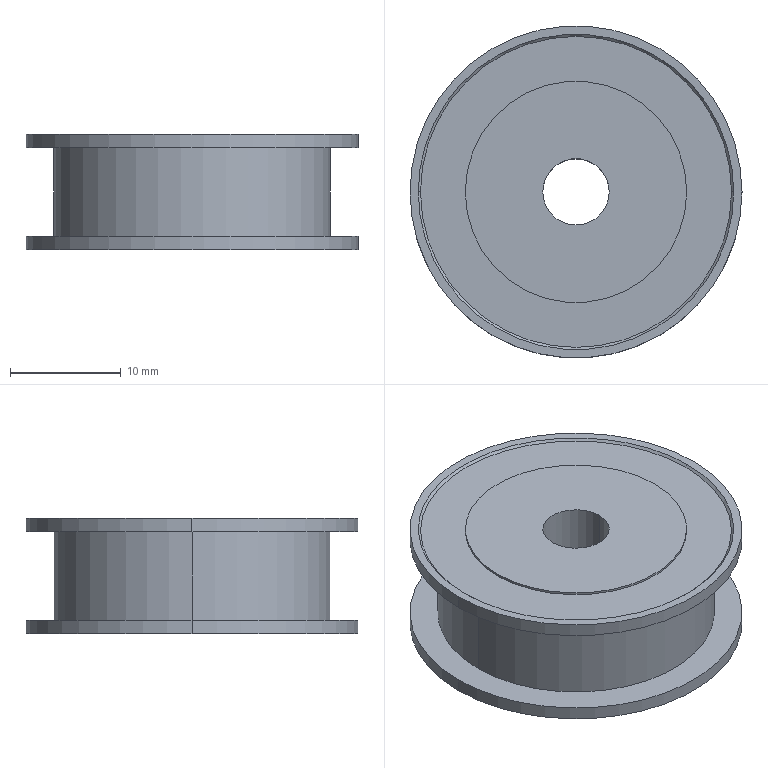Part | SolidWorks | features BaseBody 1 | 1 solid | 24 faces | box 30 x 30 x 10.4 mm | volume 5208 mm3 | cylinder 12 | plane 8 | cone 4 | commonest cylinder face diameters 20 x4 30 x4 6 x2 25 x2
STEP:
#1=CARTESIAN_POINT('',(-12.5,0.,0.));
#2=VERTEX_POINT('',#1);
#3=CARTESIAN_POINT('',(12.5,0.,0.));
#4=VERTEX_POINT('',#3);
#5=CARTESIAN_POINT('',(0.,0.,0.));
#6=DIRECTION('',(0.,0.,-1.));
#7=DIRECTION('',(-1.,0.,0.));
#8=AXIS2_PLACEMENT_3D('',#5,#6,#7);
#9=CIRCLE('',#8,12.5);
#10=EDGE_CURVE('',#2,#4,#9,.T.);
#11=ORIENTED_EDGE('',*,*,#10,.T.);
#12=CARTESIAN_POINT('',(12.5,0.,-8.));
#13=VERTEX_POINT('',#12);
#14=CARTESIAN_POINT('',(12.5,0.,0.));
#15=DIRECTION('',(0.,0.,-1.));
#16=VECTOR('',#15,1000.);
#17=LINE('',#14,#16);
#18=EDGE_CURVE('',#4,#13,#17,.T.);
#19=ORIENTED_EDGE('',*,*,#18,.T.);
#20=CARTESIAN_POINT('',(-12.5,0.,-8.));
#21=VERTEX_POINT('',#20);
#22=CARTESIAN_POINT('',(0.,0.,-8.));
#23=DIRECTION('',(0.,0.,1.));
#24=DIRECTION('',(-1.,0.,0.));
#25=AXIS2_PLACEMENT_3D('',#22,#23,#24);
#26=CIRCLE('',#25,12.5);
#27=EDGE_CURVE('',#13,#21,#26,.T.);
#28=ORIENTED_EDGE('',*,*,#27,.T.);
#29=CARTESIAN_POINT('',(-12.5,0.,0.));
#30=DIRECTION('',(0.,0.,-1.));
#31=VECTOR('',#30,1000.);
#32=LINE('',#29,#31);
#33=EDGE_CURVE('',#2,#21,#32,.T.);
#34=ORIENTED_EDGE('',*,*,#33,.F.);
#35=EDGE_LOOP('',(#11,#19,#28,#34));
#36=FACE_OUTER_BOUND('',#35,.T.);
#37=CARTESIAN_POINT('',(0.,0.,0.));
#38=DIRECTION('',(0.,0.,-1.));
#39=DIRECTION('',(-1.,0.,0.));
#40=AXIS2_PLACEMENT_3D('',#37,#38,#39);
#41=CYLINDRICAL_SURFACE('',#40,12.5);
#42=ADVANCED_FACE('',(#36),#41,.T.);
#43=CARTESIAN_POINT('',(-15.,0.,0.));
#44=VERTEX_POINT('',#43);
#45=CARTESIAN_POINT('',(15.,0.,0.));
#46=VERTEX_POINT('',#45);
#47=CARTESIAN_POINT('',(0.,0.,0.));
#48=DIRECTION('',(0.,0.,-1.));
#49=DIRECTION('',(1.,0.,0.));
#50=AXIS2_PLACEMENT_3D('',#47,#48,#49);
#51=CIRCLE('',#50,15.);
#52=EDGE_CURVE('',#44,#46,#51,.T.);
#53=ORIENTED_EDGE('',*,*,#52,.F.);
#54=CARTESIAN_POINT('',(-15.,0.,1.2));
#55=VERTEX_POINT('',#54);
#56=CARTESIAN_POINT('',(-15.,0.,0.));
#57=DIRECTION('',(0.,0.,1.));
#58=VECTOR('',#57,1000.);
#59=LINE('',#56,#58);
#60=EDGE_CURVE('',#44,#55,#59,.T.);
#61=ORIENTED_EDGE('',*,*,#60,.T.);
#62=CARTESIAN_POINT('',(15.,0.,1.2));
#63=VERTEX_POINT('',#62);
#64=CARTESIAN_POINT('',(0.,0.,1.2));
#65=DIRECTION('',(0.,0.,-1.));
#66=DIRECTION('',(1.,0.,0.));
#67=AXIS2_PLACEMENT_3D('',#64,#65,#66);
#68=CIRCLE('',#67,15.);
#69=EDGE_CURVE('',#55,#63,#68,.T.);
#70=ORIENTED_EDGE('',*,*,#69,.T.);
#71=CARTESIAN_POINT('',(15.,0.,0.));
#72=DIRECTION('',(0.,0.,1.));
#73=VECTOR('',#72,1000.);
#74=LINE('',#71,#73);
#75=EDGE_CURVE('',#46,#63,#74,.T.);
#76=ORIENTED_EDGE('',*,*,#75,.F.);
#77=EDGE_LOOP('',(#53,#61,#70,#76));
#78=FACE_OUTER_BOUND('',#77,.T.);
#79=CARTESIAN_POINT('',(0.,0.,0.));
#80=DIRECTION('',(0.,0.,1.));
#81=DIRECTION('',(1.,0.,0.));
#82=AXIS2_PLACEMENT_3D('',#79,#80,#81);
#83=CYLINDRICAL_SURFACE('',#82,15.);
#84=ADVANCED_FACE('',(#78),#83,.T.);
#85=CARTESIAN_POINT('',(15.,0.,-8.));
#86=VERTEX_POINT('',#85);
#87=CARTESIAN_POINT('',(-15.,0.,-8.));
#88=VERTEX_POINT('',#87);
#89=CARTESIAN_POINT('',(0.,0.,-8.));
#90=DIRECTION('',(0.,0.,1.));
#91=DIRECTION('',(-1.,0.,0.));
#92=AXIS2_PLACEMENT_3D('',#89,#90,#91);
#93=CIRCLE('',#92,15.);
#94=EDGE_CURVE('',#86,#88,#93,.T.);
#95=ORIENTED_EDGE('',*,*,#94,.F.);
#96=CARTESIAN_POINT('',(15.,0.,-9.2));
#97=VERTEX_POINT('',#96);
#98=CARTESIAN_POINT('',(15.,0.,-8.));
#99=DIRECTION('',(0.,0.,-1.));
#100=VECTOR('',#99,1000.);
#101=LINE('',#98,#100);
#102=EDGE_CURVE('',#86,#97,#101,.T.);
#103=ORIENTED_EDGE('',*,*,#102,.T.);
#104=CARTESIAN_POINT('',(-15.,0.,-9.2));
#105=VERTEX_POINT('',#104);
#106=CARTESIAN_POINT('',(0.,0.,-9.2));
#107=DIRECTION('',(0.,0.,1.));
#108=DIRECTION('',(-1.,0.,0.));
#109=AXIS2_PLACEMENT_3D('',#106,#107,#108);
#110=CIRCLE('',#109,15.);
#111=EDGE_CURVE('',#97,#105,#110,.T.);
#112=ORIENTED_EDGE('',*,*,#111,.T.);
#113=CARTESIAN_POINT('',(-15.,0.,-8.));
#114=DIRECTION('',(0.,0.,-1.));
#115=VECTOR('',#114,1000.);
#116=LINE('',#113,#115);
#117=EDGE_CURVE('',#88,#105,#116,.T.);
#118=ORIENTED_EDGE('',*,*,#117,.F.);
#119=EDGE_LOOP('',(#95,#103,#112,#118));
#120=FACE_OUTER_BOUND('',#119,.T.);
#121=CARTESIAN_POINT('',(0.,0.,-8.));
#122=DIRECTION('',(0.,0.,-1.));
#123=DIRECTION('',(-1.,0.,0.));
#124=AXIS2_PLACEMENT_3D('',#121,#122,#123);
#125=CYLINDRICAL_SURFACE('',#124,15.);
#126=ADVANCED_FACE('',(#120),#125,.T.);
#127=CARTESIAN_POINT('',(-14.05,0.,1.));
#128=VERTEX_POINT('',#127);
#129=CARTESIAN_POINT('',(14.05,0.,1.));
#130=VERTEX_POINT('',#129);
#131=CARTESIAN_POINT('',(0.,0.,1.));
#132=DIRECTION('',(0.,0.,1.));
#133=DIRECTION('',(1.,0.,0.));
#134=AXIS2_PLACEMENT_3D('',#131,#132,#133);
#135=CIRCLE('',#134,14.05);
#136=EDGE_CURVE('',#128,#130,#135,.T.);
#137=ORIENTED_EDGE('',*,*,#136,.F.);
#138=CARTESIAN_POINT('',(-14.25,0.,1.2));
#139=VERTEX_POINT('',#138);
#140=CARTESIAN_POINT('',(-14.25,0.,1.2));
#141=DIRECTION('',(-0.7071,0.,0.7071));
#142=VECTOR('',#141,1000.);
#143=LINE('',#140,#142);
#144=EDGE_CURVE('',#128,#139,#143,.T.);
#145=ORIENTED_EDGE('',*,*,#144,.T.);
#146=CARTESIAN_POINT('',(14.25,0.,1.2));
#147=VERTEX_POINT('',#146);
#148=CARTESIAN_POINT('',(0.,0.,1.2));
#149=DIRECTION('',(0.,0.,1.));
#150=DIRECTION('',(1.,0.,0.));
#151=AXIS2_PLACEMENT_3D('',#148,#149,#150);
#152=CIRCLE('',#151,14.25);
#153=EDGE_CURVE('',#139,#147,#152,.T.);
#154=ORIENTED_EDGE('',*,*,#153,.T.);
#155=CARTESIAN_POINT('',(14.25,0.,1.2));
#156=DIRECTION('',(0.7071,0.,0.7071));
#157=VECTOR('',#156,1000.);
#158=LINE('',#155,#157);
#159=EDGE_CURVE('',#130,#147,#158,.T.);
#160=ORIENTED_EDGE('',*,*,#159,.F.);
#161=EDGE_LOOP('',(#137,#145,#154,#160));
#162=FACE_OUTER_BOUND('',#161,.T.);
#163=CARTESIAN_POINT('',(0.,0.,1.2));
#164=DIRECTION('',(0.,0.,1.));
#165=DIRECTION('',(1.,0.,0.));
#166=AXIS2_PLACEMENT_3D('',#163,#164,#165);
#167=CONICAL_SURFACE('',#166,14.25,0.7854);
#168=ADVANCED_FACE('',(#162),#167,.F.);
#169=CARTESIAN_POINT('',(0.,-13.8,-9.));
#170=VERTEX_POINT('',#169);
#171=CARTESIAN_POINT('',(0.,13.8,-9.));
#172=VERTEX_POINT('',#171);
#173=CARTESIAN_POINT('',(0.,0.,-9.));
#174=DIRECTION('',(0.,0.,-1.));
#175=DIRECTION('',(0.,1.,0.));
#176=AXIS2_PLACEMENT_3D('',#173,#174,#175);
#177=CIRCLE('',#176,13.8);
#178=EDGE_CURVE('',#170,#172,#177,.T.);
#179=ORIENTED_EDGE('',*,*,#178,.F.);
#180=CARTESIAN_POINT('',(0.,-14.,-9.2));
#181=VERTEX_POINT('',#180);
#182=CARTESIAN_POINT('',(0.,-14.,-9.2));
#183=DIRECTION('',(0.,-0.7071,-0.7071));
#184=VECTOR('',#183,1000.);
#185=LINE('',#182,#184);
#186=EDGE_CURVE('',#170,#181,#185,.T.);
#187=ORIENTED_EDGE('',*,*,#186,.T.);
#188=CARTESIAN_POINT('',(0.,14.,-9.2));
#189=VERTEX_POINT('',#188);
#190=CARTESIAN_POINT('',(0.,0.,-9.2));
#191=DIRECTION('',(0.,0.,-1.));
#192=DIRECTION('',(0.,1.,0.));
#193=AXIS2_PLACEMENT_3D('',#190,#191,#192);
#194=CIRCLE('',#193,14.);
#195=EDGE_CURVE('',#181,#189,#194,.T.);
#196=ORIENTED_EDGE('',*,*,#195,.T.);
#197=CARTESIAN_POINT('',(0.,14.,-9.2));
#198=DIRECTION('',(0.,0.7071,-0.7071));
#199=VECTOR('',#198,1000.);
#200=LINE('',#197,#199);
#201=EDGE_CURVE('',#172,#189,#200,.T.);
#202=ORIENTED_EDGE('',*,*,#201,.F.);
#203=EDGE_LOOP('',(#179,#187,#196,#202));
#204=FACE_OUTER_BOUND('',#203,.T.);
#205=CARTESIAN_POINT('',(0.,0.,-9.2));
#206=DIRECTION('',(0.,0.,-1.));
#207=DIRECTION('',(0.,1.,0.));
#208=AXIS2_PLACEMENT_3D('',#205,#206,#207);
#209=CONICAL_SURFACE('',#208,14.,0.7854);
#210=ADVANCED_FACE('',(#204),#209,.F.);
#211=CARTESIAN_POINT('',(10.,0.,1.));
#212=VERTEX_POINT('',#211);
#213=CARTESIAN_POINT('',(-10.,0.,1.));
#214=VERTEX_POINT('',#213);
#215=CARTESIAN_POINT('',(0.,0.,1.));
#216=DIRECTION('',(0.,0.,1.));
#217=DIRECTION('',(1.,0.,0.));
#218=AXIS2_PLACEMENT_3D('',#215,#216,#217);
#219=CIRCLE('',#218,10.);
#220=EDGE_CURVE('',#212,#214,#219,.T.);
#221=ORIENTED_EDGE('',*,*,#220,.T.);
#222=CARTESIAN_POINT('',(-10.,0.,1.2));
#223=VERTEX_POINT('',#222);
#224=CARTESIAN_POINT('',(-10.,0.,1.));
#225=DIRECTION('',(0.,0.,1.));
#226=VECTOR('',#225,1000.);
#227=LINE('',#224,#226);
#228=EDGE_CURVE('',#214,#223,#227,.T.);
#229=ORIENTED_EDGE('',*,*,#228,.T.);
#230=CARTESIAN_POINT('',(10.,0.,1.2));
#231=VERTEX_POINT('',#230);
#232=CARTESIAN_POINT('',(0.,0.,1.2));
#233=DIRECTION('',(0.,0.,-1.));
#234=DIRECTION('',(1.,0.,0.));
#235=AXIS2_PLACEMENT_3D('',#232,#233,#234);
#236=CIRCLE('',#235,10.);
#237=EDGE_CURVE('',#223,#231,#236,.T.);
#238=ORIENTED_EDGE('',*,*,#237,.T.);
#239=CARTESIAN_POINT('',(10.,0.,1.));
#240=DIRECTION('',(0.,0.,1.));
#241=VECTOR('',#240,1000.);
#242=LINE('',#239,#241);
#243=EDGE_CURVE('',#212,#231,#242,.T.);
#244=ORIENTED_EDGE('',*,*,#243,.F.);
#245=EDGE_LOOP('',(#221,#229,#238,#244));
#246=FACE_OUTER_BOUND('',#245,.T.);
#247=CARTESIAN_POINT('',(0.,0.,1.));
#248=DIRECTION('',(0.,0.,1.));
#249=DIRECTION('',(1.,0.,0.));
#250=AXIS2_PLACEMENT_3D('',#247,#248,#249);
#251=CYLINDRICAL_SURFACE('',#250,10.);
#252=ADVANCED_FACE('',(#246),#251,.T.);
#253=CARTESIAN_POINT('',(-10.,0.,-9.));
#254=VERTEX_POINT('',#253);
#255=CARTESIAN_POINT('',(10.,0.,-9.));
#256=VERTEX_POINT('',#255);
#257=CARTESIAN_POINT('',(0.,0.,-9.));
#258=DIRECTION('',(0.,0.,-1.));
#259=DIRECTION('',(-1.,0.,0.));
#260=AXIS2_PLACEMENT_3D('',#257,#258,#259);
#261=CIRCLE('',#260,10.);
#262=EDGE_CURVE('',#254,#256,#261,.T.);
#263=ORIENTED_EDGE('',*,*,#262,.T.);
#264=CARTESIAN_POINT('',(10.,0.,-9.2));
#265=VERTEX_POINT('',#264);
#266=CARTESIAN_POINT('',(10.,0.,-9.));
#267=DIRECTION('',(0.,0.,-1.));
#268=VECTOR('',#267,1000.);
#269=LINE('',#266,#268);
#270=EDGE_CURVE('',#256,#265,#269,.T.);
#271=ORIENTED_EDGE('',*,*,#270,.T.);
#272=CARTESIAN_POINT('',(-10.,0.,-9.2));
#273=VERTEX_POINT('',#272);
#274=CARTESIAN_POINT('',(0.,0.,-9.2));
#275=DIRECTION('',(0.,0.,1.));
#276=DIRECTION('',(-1.,0.,0.));
#277=AXIS2_PLACEMENT_3D('',#274,#275,#276);
#278=CIRCLE('',#277,10.);
#279=EDGE_CURVE('',#265,#273,#278,.T.);
#280=ORIENTED_EDGE('',*,*,#279,.T.);
#281=CARTESIAN_POINT('',(-10.,0.,-9.));
#282=DIRECTION('',(0.,0.,-1.));
#283=VECTOR('',#282,1000.);
#284=LINE('',#281,#283);
#285=EDGE_CURVE('',#254,#273,#284,.T.);
#286=ORIENTED_EDGE('',*,*,#285,.F.);
#287=EDGE_LOOP('',(#263,#271,#280,#286));
#288=FACE_OUTER_BOUND('',#287,.T.);
#289=CARTESIAN_POINT('',(0.,0.,-9.));
#290=DIRECTION('',(0.,0.,-1.));
#291=DIRECTION('',(-1.,0.,0.));
#292=AXIS2_PLACEMENT_3D('',#289,#290,#291);
#293=CYLINDRICAL_SURFACE('',#292,10.);
#294=ADVANCED_FACE('',(#288),#293,.T.);
#295=CARTESIAN_POINT('',(-3.,0.,1.2));
#296=VERTEX_POINT('',#295);
#297=CARTESIAN_POINT('',(3.,0.,1.2));
#298=VERTEX_POINT('',#297);
#299=CARTESIAN_POINT('',(0.,0.,1.2));
#300=DIRECTION('',(0.,0.,1.));
#301=DIRECTION('',(-1.,0.,0.));
#302=AXIS2_PLACEMENT_3D('',#299,#300,#301);
#303=CIRCLE('',#302,3.);
#304=EDGE_CURVE('',#296,#298,#303,.T.);
#305=ORIENTED_EDGE('',*,*,#304,.T.);
#306=CARTESIAN_POINT('',(3.,0.,-9.2));
#307=VERTEX_POINT('',#306);
#308=CARTESIAN_POINT('',(3.,0.,1.));
#309=DIRECTION('',(0.,0.,-1.));
#310=VECTOR('',#309,1000.);
#311=LINE('',#308,#310);
#312=EDGE_CURVE('',#298,#307,#311,.T.);
#313=ORIENTED_EDGE('',*,*,#312,.T.);
#314=CARTESIAN_POINT('',(-3.,0.,-9.2));
#315=VERTEX_POINT('',#314);
#316=CARTESIAN_POINT('',(0.,0.,-9.2));
#317=DIRECTION('',(0.,0.,-1.));
#318=DIRECTION('',(-1.,0.,0.));
#319=AXIS2_PLACEMENT_3D('',#316,#317,#318);
#320=CIRCLE('',#319,3.);
#321=EDGE_CURVE('',#307,#315,#320,.T.);
#322=ORIENTED_EDGE('',*,*,#321,.T.);
#323=CARTESIAN_POINT('',(-3.,0.,1.));
#324=DIRECTION('',(0.,0.,-1.));
#325=VECTOR('',#324,1000.);
#326=LINE('',#323,#325);
#327=EDGE_CURVE('',#296,#315,#326,.T.);
#328=ORIENTED_EDGE('',*,*,#327,.F.);
#329=EDGE_LOOP('',(#305,#313,#322,#328));
#330=FACE_OUTER_BOUND('',#329,.T.);
#331=CARTESIAN_POINT('',(0.,0.,1.));
#332=DIRECTION('',(0.,0.,-1.));
#333=DIRECTION('',(-1.,0.,0.));
#334=AXIS2_PLACEMENT_3D('',#331,#332,#333);
#335=CYLINDRICAL_SURFACE('',#334,3.);
#336=ADVANCED_FACE('',(#330),#335,.F.);
#337=ORIENTED_EDGE('',*,*,#18,.F.);
#338=CARTESIAN_POINT('',(0.,0.,0.));
#339=DIRECTION('',(0.,0.,-1.));
#340=DIRECTION('',(-1.,0.,0.));
#341=AXIS2_PLACEMENT_3D('',#338,#339,#340);
#342=CIRCLE('',#341,12.5);
#343=EDGE_CURVE('',#4,#2,#342,.T.);
#344=ORIENTED_EDGE('',*,*,#343,.T.);
#345=ORIENTED_EDGE('',*,*,#33,.T.);
#346=CARTESIAN_POINT('',(0.,0.,-8.));
#347=DIRECTION('',(0.,0.,1.));
#348=DIRECTION('',(-1.,0.,0.));
#349=AXIS2_PLACEMENT_3D('',#346,#347,#348);
#350=CIRCLE('',#349,12.5);
#351=EDGE_CURVE('',#21,#13,#350,.T.);
#352=ORIENTED_EDGE('',*,*,#351,.T.);
#353=EDGE_LOOP('',(#337,#344,#345,#352));
#354=FACE_OUTER_BOUND('',#353,.T.);
#355=CARTESIAN_POINT('',(0.,0.,0.));
#356=DIRECTION('',(0.,0.,-1.));
#357=DIRECTION('',(-1.,0.,0.));
#358=AXIS2_PLACEMENT_3D('',#355,#356,#357);
#359=CYLINDRICAL_SURFACE('',#358,12.5);
#360=ADVANCED_FACE('',(#354),#359,.T.);
#361=ORIENTED_EDGE('',*,*,#10,.F.);
#362=ORIENTED_EDGE('',*,*,#343,.F.);
#363=EDGE_LOOP('',(#361,#362));
#364=FACE_BOUND('',#363,.T.);
#365=CARTESIAN_POINT('',(0.,0.,0.));
#366=DIRECTION('',(0.,0.,-1.));
#367=DIRECTION('',(1.,0.,0.));
#368=AXIS2_PLACEMENT_3D('',#365,#366,#367);
#369=CIRCLE('',#368,15.);
#370=EDGE_CURVE('',#46,#44,#369,.T.);
#371=ORIENTED_EDGE('',*,*,#370,.T.);
#372=ORIENTED_EDGE('',*,*,#52,.T.);
#373=EDGE_LOOP('',(#371,#372));
#374=FACE_OUTER_BOUND('',#373,.T.);
#375=CARTESIAN_POINT('',(0.,0.,0.));
#376=DIRECTION('',(0.,0.,-1.));
#377=DIRECTION('',(-1.,0.,0.));
#378=AXIS2_PLACEMENT_3D('',#375,#376,#377);
#379=PLANE('',#378);
#380=ADVANCED_FACE('',(#364,#374),#379,.T.);
#381=ORIENTED_EDGE('',*,*,#351,.F.);
#382=ORIENTED_EDGE('',*,*,#27,.F.);
#383=EDGE_LOOP('',(#381,#382));
#384=FACE_BOUND('',#383,.T.);
#385=CARTESIAN_POINT('',(0.,0.,-8.));
#386=DIRECTION('',(0.,0.,1.));
#387=DIRECTION('',(-1.,0.,0.));
#388=AXIS2_PLACEMENT_3D('',#385,#386,#387);
#389=CIRCLE('',#388,15.);
#390=EDGE_CURVE('',#88,#86,#389,.T.);
#391=ORIENTED_EDGE('',*,*,#390,.T.);
#392=ORIENTED_EDGE('',*,*,#94,.T.);
#393=EDGE_LOOP('',(#391,#392));
#394=FACE_OUTER_BOUND('',#393,.T.);
#395=CARTESIAN_POINT('',(0.,0.,-8.));
#396=DIRECTION('',(0.,0.,1.));
#397=DIRECTION('',(1.,0.,0.));
#398=AXIS2_PLACEMENT_3D('',#395,#396,#397);
#399=PLANE('',#398);
#400=ADVANCED_FACE('',(#384,#394),#399,.T.);
#401=ORIENTED_EDGE('',*,*,#60,.F.);
#402=ORIENTED_EDGE('',*,*,#370,.F.);
#403=ORIENTED_EDGE('',*,*,#75,.T.);
#404=CARTESIAN_POINT('',(0.,0.,1.2));
#405=DIRECTION('',(0.,0.,-1.));
#406=DIRECTION('',(1.,0.,0.));
#407=AXIS2_PLACEMENT_3D('',#404,#405,#406);
#408=CIRCLE('',#407,15.);
#409=EDGE_CURVE('',#63,#55,#408,.T.);
#410=ORIENTED_EDGE('',*,*,#409,.T.);
#411=EDGE_LOOP('',(#401,#402,#403,#410));
#412=FACE_OUTER_BOUND('',#411,.T.);
#413=CARTESIAN_POINT('',(0.,0.,0.));
#414=DIRECTION('',(0.,0.,1.));
#415=DIRECTION('',(1.,0.,0.));
#416=AXIS2_PLACEMENT_3D('',#413,#414,#415);
#417=CYLINDRICAL_SURFACE('',#416,15.);
#418=ADVANCED_FACE('',(#412),#417,.T.);
#419=ORIENTED_EDGE('',*,*,#102,.F.);
#420=ORIENTED_EDGE('',*,*,#390,.F.);
#421=ORIENTED_EDGE('',*,*,#117,.T.);
#422=CARTESIAN_POINT('',(0.,0.,-9.2));
#423=DIRECTION('',(0.,0.,1.));
#424=DIRECTION('',(-1.,0.,0.));
#425=AXIS2_PLACEMENT_3D('',#422,#423,#424);
#426=CIRCLE('',#425,15.);
#427=EDGE_CURVE('',#105,#97,#426,.T.);
#428=ORIENTED_EDGE('',*,*,#427,.T.);
#429=EDGE_LOOP('',(#419,#420,#421,#428));
#430=FACE_OUTER_BOUND('',#429,.T.);
#431=CARTESIAN_POINT('',(0.,0.,-8.));
#432=DIRECTION('',(0.,0.,-1.));
#433=DIRECTION('',(-1.,0.,0.));
#434=AXIS2_PLACEMENT_3D('',#431,#432,#433);
#435=CYLINDRICAL_SURFACE('',#434,15.);
#436=ADVANCED_FACE('',(#430),#435,.T.);
#437=CARTESIAN_POINT('',(0.,0.,1.2));
#438=DIRECTION('',(0.,0.,1.));
#439=DIRECTION('',(1.,0.,0.));
#440=AXIS2_PLACEMENT_3D('',#437,#438,#439);
#441=CIRCLE('',#440,14.25);
#442=EDGE_CURVE('',#147,#139,#441,.T.);
#443=ORIENTED_EDGE('',*,*,#442,.F.);
#444=ORIENTED_EDGE('',*,*,#153,.F.);
#445=EDGE_LOOP('',(#443,#444));
#446=FACE_BOUND('',#445,.T.);
#447=ORIENTED_EDGE('',*,*,#409,.F.);
#448=ORIENTED_EDGE('',*,*,#69,.F.);
#449=EDGE_LOOP('',(#447,#448));
#450=FACE_OUTER_BOUND('',#449,.T.);
#451=CARTESIAN_POINT('',(0.,0.,1.2));
#452=DIRECTION('',(0.,0.,-1.));
#453=DIRECTION('',(-1.,0.,0.));
#454=AXIS2_PLACEMENT_3D('',#451,#452,#453);
#455=PLANE('',#454);
#456=ADVANCED_FACE('',(#446,#450),#455,.F.);
#457=CARTESIAN_POINT('',(0.,0.,-9.2));
#458=DIRECTION('',(0.,0.,-1.));
#459=DIRECTION('',(0.,1.,0.));
#460=AXIS2_PLACEMENT_3D('',#457,#458,#459);
#461=CIRCLE('',#460,14.);
#462=EDGE_CURVE('',#189,#181,#461,.T.);
#463=ORIENTED_EDGE('',*,*,#462,.F.);
#464=ORIENTED_EDGE('',*,*,#195,.F.);
#465=EDGE_LOOP('',(#463,#464));
#466=FACE_BOUND('',#465,.T.);
#467=ORIENTED_EDGE('',*,*,#427,.F.);
#468=ORIENTED_EDGE('',*,*,#111,.F.);
#469=EDGE_LOOP('',(#467,#468));
#470=FACE_OUTER_BOUND('',#469,.T.);
#471=CARTESIAN_POINT('',(0.,0.,-9.2));
#472=DIRECTION('',(0.,0.,1.));
#473=DIRECTION('',(1.,0.,0.));
#474=AXIS2_PLACEMENT_3D('',#471,#472,#473);
#475=PLANE('',#474);
#476=ADVANCED_FACE('',(#466,#470),#475,.F.);
#477=ORIENTED_EDGE('',*,*,#144,.F.);
#478=CARTESIAN_POINT('',(0.,0.,1.));
#479=DIRECTION('',(0.,0.,1.));
#480=DIRECTION('',(1.,0.,0.));
#481=AXIS2_PLACEMENT_3D('',#478,#479,#480);
#482=CIRCLE('',#481,14.05);
#483=EDGE_CURVE('',#130,#128,#482,.T.);
#484=ORIENTED_EDGE('',*,*,#483,.F.);
#485=ORIENTED_EDGE('',*,*,#159,.T.);
#486=ORIENTED_EDGE('',*,*,#442,.T.);
#487=EDGE_LOOP('',(#477,#484,#485,#486));
#488=FACE_OUTER_BOUND('',#487,.T.);
#489=CARTESIAN_POINT('',(0.,0.,1.2));
#490=DIRECTION('',(0.,0.,1.));
#491=DIRECTION('',(1.,0.,0.));
#492=AXIS2_PLACEMENT_3D('',#489,#490,#491);
#493=CONICAL_SURFACE('',#492,14.25,0.7854);
#494=ADVANCED_FACE('',(#488),#493,.F.);
#495=ORIENTED_EDGE('',*,*,#186,.F.);
#496=CARTESIAN_POINT('',(0.,0.,-9.));
#497=DIRECTION('',(0.,0.,-1.));
#498=DIRECTION('',(0.,1.,0.));
#499=AXIS2_PLACEMENT_3D('',#496,#497,#498);
#500=CIRCLE('',#499,13.8);
#501=EDGE_CURVE('',#172,#170,#500,.T.);
#502=ORIENTED_EDGE('',*,*,#501,.F.);
#503=ORIENTED_EDGE('',*,*,#201,.T.);
#504=ORIENTED_EDGE('',*,*,#462,.T.);
#505=EDGE_LOOP('',(#495,#502,#503,#504));
#506=FACE_OUTER_BOUND('',#505,.T.);
#507=CARTESIAN_POINT('',(0.,0.,-9.2));
#508=DIRECTION('',(0.,0.,-1.));
#509=DIRECTION('',(0.,1.,0.));
#510=AXIS2_PLACEMENT_3D('',#507,#508,#509);
#511=CONICAL_SURFACE('',#510,14.,0.7854);
#512=ADVANCED_FACE('',(#506),#511,.F.);
#513=ORIENTED_EDGE('',*,*,#220,.F.);
#514=CARTESIAN_POINT('',(0.,0.,1.));
#515=DIRECTION('',(0.,0.,1.));
#516=DIRECTION('',(1.,0.,0.));
#517=AXIS2_PLACEMENT_3D('',#514,#515,#516);
#518=CIRCLE('',#517,10.);
#519=EDGE_CURVE('',#214,#212,#518,.T.);
#520=ORIENTED_EDGE('',*,*,#519,.F.);
#521=EDGE_LOOP('',(#513,#520));
#522=FACE_BOUND('',#521,.T.);
#523=ORIENTED_EDGE('',*,*,#483,.T.);
#524=ORIENTED_EDGE('',*,*,#136,.T.);
#525=EDGE_LOOP('',(#523,#524));
#526=FACE_OUTER_BOUND('',#525,.T.);
#527=CARTESIAN_POINT('',(0.,0.,1.));
#528=DIRECTION('',(0.,0.,-1.));
#529=DIRECTION('',(-1.,0.,0.));
#530=AXIS2_PLACEMENT_3D('',#527,#528,#529);
#531=PLANE('',#530);
#532=ADVANCED_FACE('',(#522,#526),#531,.F.);
#533=ORIENTED_EDGE('',*,*,#262,.F.);
#534=CARTESIAN_POINT('',(0.,0.,-9.));
#535=DIRECTION('',(0.,0.,-1.));
#536=DIRECTION('',(-1.,0.,0.));
#537=AXIS2_PLACEMENT_3D('',#534,#535,#536);
#538=CIRCLE('',#537,10.);
#539=EDGE_CURVE('',#256,#254,#538,.T.);
#540=ORIENTED_EDGE('',*,*,#539,.F.);
#541=EDGE_LOOP('',(#533,#540));
#542=FACE_BOUND('',#541,.T.);
#543=ORIENTED_EDGE('',*,*,#501,.T.);
#544=ORIENTED_EDGE('',*,*,#178,.T.);
#545=EDGE_LOOP('',(#543,#544));
#546=FACE_OUTER_BOUND('',#545,.T.);
#547=CARTESIAN_POINT('',(0.,0.,-9.));
#548=DIRECTION('',(0.,0.,1.));
#549=DIRECTION('',(1.,0.,0.));
#550=AXIS2_PLACEMENT_3D('',#547,#548,#549);
#551=PLANE('',#550);
#552=ADVANCED_FACE('',(#542,#546),#551,.F.);
#553=ORIENTED_EDGE('',*,*,#228,.F.);
#554=ORIENTED_EDGE('',*,*,#519,.T.);
#555=ORIENTED_EDGE('',*,*,#243,.T.);
#556=CARTESIAN_POINT('',(0.,0.,1.2));
#557=DIRECTION('',(0.,0.,-1.));
#558=DIRECTION('',(1.,0.,0.));
#559=AXIS2_PLACEMENT_3D('',#556,#557,#558);
#560=CIRCLE('',#559,10.);
#561=EDGE_CURVE('',#231,#223,#560,.T.);
#562=ORIENTED_EDGE('',*,*,#561,.T.);
#563=EDGE_LOOP('',(#553,#554,#555,#562));
#564=FACE_OUTER_BOUND('',#563,.T.);
#565=CARTESIAN_POINT('',(0.,0.,1.));
#566=DIRECTION('',(0.,0.,1.));
#567=DIRECTION('',(1.,0.,0.));
#568=AXIS2_PLACEMENT_3D('',#565,#566,#567);
#569=CYLINDRICAL_SURFACE('',#568,10.);
#570=ADVANCED_FACE('',(#564),#569,.T.);
#571=ORIENTED_EDGE('',*,*,#270,.F.);
#572=ORIENTED_EDGE('',*,*,#539,.T.);
#573=ORIENTED_EDGE('',*,*,#285,.T.);
#574=CARTESIAN_POINT('',(0.,0.,-9.2));
#575=DIRECTION('',(0.,0.,1.));
#576=DIRECTION('',(-1.,0.,0.));
#577=AXIS2_PLACEMENT_3D('',#574,#575,#576);
#578=CIRCLE('',#577,10.);
#579=EDGE_CURVE('',#273,#265,#578,.T.);
#580=ORIENTED_EDGE('',*,*,#579,.T.);
#581=EDGE_LOOP('',(#571,#572,#573,#580));
#582=FACE_OUTER_BOUND('',#581,.T.);
#583=CARTESIAN_POINT('',(0.,0.,-9.));
#584=DIRECTION('',(0.,0.,-1.));
#585=DIRECTION('',(-1.,0.,0.));
#586=AXIS2_PLACEMENT_3D('',#583,#584,#585);
#587=CYLINDRICAL_SURFACE('',#586,10.);
#588=ADVANCED_FACE('',(#582),#587,.T.);
#589=ORIENTED_EDGE('',*,*,#304,.F.);
#590=CARTESIAN_POINT('',(0.,0.,1.2));
#591=DIRECTION('',(0.,0.,1.));
#592=DIRECTION('',(-1.,0.,0.));
#593=AXIS2_PLACEMENT_3D('',#590,#591,#592);
#594=CIRCLE('',#593,3.);
#595=EDGE_CURVE('',#298,#296,#594,.T.);
#596=ORIENTED_EDGE('',*,*,#595,.F.);
#597=EDGE_LOOP('',(#589,#596));
#598=FACE_BOUND('',#597,.T.);
#599=ORIENTED_EDGE('',*,*,#561,.F.);
#600=ORIENTED_EDGE('',*,*,#237,.F.);
#601=EDGE_LOOP('',(#599,#600));
#602=FACE_OUTER_BOUND('',#601,.T.);
#603=CARTESIAN_POINT('',(0.,0.,1.2));
#604=DIRECTION('',(0.,0.,-1.));
#605=DIRECTION('',(-1.,0.,0.));
#606=AXIS2_PLACEMENT_3D('',#603,#604,#605);
#607=PLANE('',#606);
#608=ADVANCED_FACE('',(#598,#602),#607,.F.);
#609=CARTESIAN_POINT('',(0.,0.,-9.2));
#610=DIRECTION('',(0.,0.,-1.));
#611=DIRECTION('',(-1.,0.,0.));
#612=AXIS2_PLACEMENT_3D('',#609,#610,#611);
#613=CIRCLE('',#612,3.);
#614=EDGE_CURVE('',#315,#307,#613,.T.);
#615=ORIENTED_EDGE('',*,*,#614,.F.);
#616=ORIENTED_EDGE('',*,*,#321,.F.);
#617=EDGE_LOOP('',(#615,#616));
#618=FACE_BOUND('',#617,.T.);
#619=ORIENTED_EDGE('',*,*,#579,.F.);
#620=ORIENTED_EDGE('',*,*,#279,.F.);
#621=EDGE_LOOP('',(#619,#620));
#622=FACE_OUTER_BOUND('',#621,.T.);
#623=CARTESIAN_POINT('',(0.,0.,-9.2));
#624=DIRECTION('',(0.,0.,1.));
#625=DIRECTION('',(1.,0.,0.));
#626=AXIS2_PLACEMENT_3D('',#623,#624,#625);
#627=PLANE('',#626);
#628=ADVANCED_FACE('',(#618,#622),#627,.F.);
#629=ORIENTED_EDGE('',*,*,#312,.F.);
#630=ORIENTED_EDGE('',*,*,#595,.T.);
#631=ORIENTED_EDGE('',*,*,#327,.T.);
#632=ORIENTED_EDGE('',*,*,#614,.T.);
#633=EDGE_LOOP('',(#629,#630,#631,#632));
#634=FACE_OUTER_BOUND('',#633,.T.);
#635=CARTESIAN_POINT('',(0.,0.,1.));
#636=DIRECTION('',(0.,0.,-1.));
#637=DIRECTION('',(-1.,0.,0.));
#638=AXIS2_PLACEMENT_3D('',#635,#636,#637);
#639=CYLINDRICAL_SURFACE('',#638,3.);
#640=ADVANCED_FACE('',(#634),#639,.F.);
#641=CLOSED_SHELL('',(#42,#84,#126,#168,#210,#252,#294,#336,#360,#380,#400,#418,#436,#456,#476,#494,#512,#532,#552,#570,#588,#608,#628,#640));
#642=MANIFOLD_SOLID_BREP('',#641);
#643=CARTESIAN_POINT('',(0.,0.,0.));
#644=DIRECTION('',(0.,0.,1.));
#645=DIRECTION('',(1.,0.,0.));
#646=AXIS2_PLACEMENT_3D('',#643,#644,#645);
#647=(LENGTH_UNIT()NAMED_UNIT(*)SI_UNIT(.MILLI.,.METRE.));
#648=UNCERTAINTY_MEASURE_WITH_UNIT(LENGTH_MEASURE(0.00001),#647,'','');
#649=(NAMED_UNIT(*)PLANE_ANGLE_UNIT()SI_UNIT($,.RADIAN.));
#650=(NAMED_UNIT(*)SI_UNIT($,.STERADIAN.)SOLID_ANGLE_UNIT());
#651=(GEOMETRIC_REPRESENTATION_CONTEXT(3)GLOBAL_UNCERTAINTY_ASSIGNED_CONTEXT((#648))GLOBAL_UNIT_ASSIGNED_CONTEXT((#647,#649,#650))REPRESENTATION_CONTEXT('',''));
#652=ADVANCED_BREP_SHAPE_REPRESENTATION('',(#642,#646),#651);